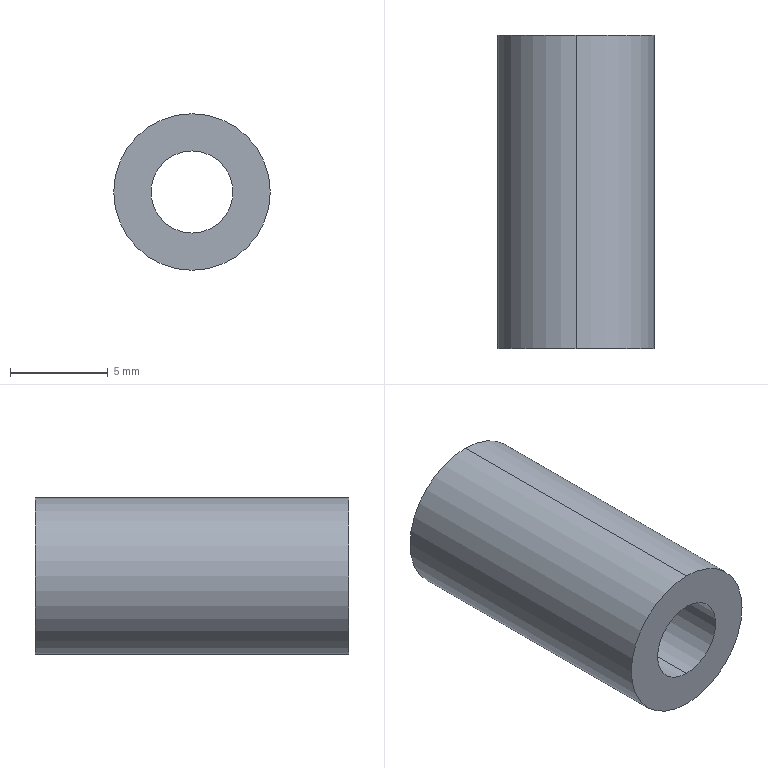Part | STEP file | 1 solid | 6 faces | box 8 x 16 x 8 mm | volume 582.577 mm3 | cylinder 4 | plane 2 | commonest cylinder face diameters 4.2 x2 8 x2
STEP:
#1=CARTESIAN_POINT('',(0.,0.,0.));
#2=DIRECTION('',(0.,0.,1.));
#3=DIRECTION('',(1.,0.,0.));
#4=AXIS2_PLACEMENT_3D('',#1,#2,#3);
#5=CARTESIAN_POINT('',(0.,16.,-2.1));
#6=VERTEX_POINT('',#5);
#7=CARTESIAN_POINT('',(0.,0.,-2.1));
#8=VERTEX_POINT('',#7);
#9=CARTESIAN_POINT('',(0.,16.,-2.1));
#10=DIRECTION('',(0.,-1.,0.));
#11=VECTOR('',#10,1.);
#12=LINE('',#9,#11);
#13=CARTESIAN_POINT('',(0.,16.,0.));
#14=DIRECTION('',(0.,-1.,0.));
#15=DIRECTION('',(0.,0.,-1.));
#16=AXIS2_PLACEMENT_3D('',#13,#14,#15);
#17=CYLINDRICAL_SURFACE('',#16,2.1);
#18=CARTESIAN_POINT('',(6.283,0.));
#19=DIRECTION('',(0.,1.));
#20=VECTOR('',#19,1.);
#21=LINE('',#18,#20);
#22=(GEOMETRIC_REPRESENTATION_CONTEXT(2)PARAMETRIC_REPRESENTATION_CONTEXT()REPRESENTATION_CONTEXT('',''));
#23=DEFINITIONAL_REPRESENTATION('',(#21),#22);
#24=PCURVE('',#17,#23);
#25=CARTESIAN_POINT('',(0.,16.,0.));
#26=DIRECTION('',(0.,-1.,0.));
#27=DIRECTION('',(0.,0.,-1.));
#28=AXIS2_PLACEMENT_3D('',#25,#26,#27);
#29=CYLINDRICAL_SURFACE('',#28,2.1);
#30=CARTESIAN_POINT('',(0.,0.));
#31=DIRECTION('',(0.,1.));
#32=VECTOR('',#31,1.);
#33=LINE('',#30,#32);
#34=(GEOMETRIC_REPRESENTATION_CONTEXT(2)PARAMETRIC_REPRESENTATION_CONTEXT()REPRESENTATION_CONTEXT('',''));
#35=DEFINITIONAL_REPRESENTATION('',(#33),#34);
#36=PCURVE('',#29,#35);
#37=SURFACE_CURVE('',#12,(#24,#36),.PCURVE_S1.);
#38=EDGE_CURVE('',#6,#8,#37,.T.);
#39=ORIENTED_EDGE('',*,*,#38,.T.);
#40=CARTESIAN_POINT('',(0.,0.,2.1));
#41=VERTEX_POINT('',#40);
#42=CARTESIAN_POINT('',(0.,0.,0.));
#43=DIRECTION('',(0.,1.,0.));
#44=DIRECTION('',(0.,0.,1.));
#45=AXIS2_PLACEMENT_3D('',#42,#43,#44);
#46=CIRCLE('',#45,2.1);
#47=CARTESIAN_POINT('',(9.425,16.));
#48=DIRECTION('',(-1.,0.));
#49=VECTOR('',#48,1.);
#50=LINE('',#47,#49);
#51=(GEOMETRIC_REPRESENTATION_CONTEXT(2)PARAMETRIC_REPRESENTATION_CONTEXT()REPRESENTATION_CONTEXT('',''));
#52=DEFINITIONAL_REPRESENTATION('',(#50),#51);
#53=PCURVE('',#17,#52);
#54=CARTESIAN_POINT('',(0.,0.,0.));
#55=DIRECTION('',(0.,1.,0.));
#56=DIRECTION('',(0.,0.,1.));
#57=AXIS2_PLACEMENT_3D('',#54,#55,#56);
#58=PLANE('',#57);
#59=CARTESIAN_POINT('',(0.,0.));
#60=DIRECTION('',(1.,0.));
#61=AXIS2_PLACEMENT_2D('',#59,#60);
#62=CIRCLE('',#61,2.1);
#63=(GEOMETRIC_REPRESENTATION_CONTEXT(2)PARAMETRIC_REPRESENTATION_CONTEXT()REPRESENTATION_CONTEXT('',''));
#64=DEFINITIONAL_REPRESENTATION('',(#62),#63);
#65=PCURVE('',#58,#64);
#66=SURFACE_CURVE('',#46,(#53,#65),.PCURVE_S1.);
#67=EDGE_CURVE('',#8,#41,#66,.T.);
#68=ORIENTED_EDGE('',*,*,#67,.T.);
#69=CARTESIAN_POINT('',(0.,16.,2.1));
#70=VERTEX_POINT('',#69);
#71=CARTESIAN_POINT('',(0.,16.,2.1));
#72=DIRECTION('',(0.,-1.,0.));
#73=VECTOR('',#72,1.);
#74=LINE('',#71,#73);
#75=CARTESIAN_POINT('',(3.142,0.));
#76=DIRECTION('',(0.,1.));
#77=VECTOR('',#76,1.);
#78=LINE('',#75,#77);
#79=(GEOMETRIC_REPRESENTATION_CONTEXT(2)PARAMETRIC_REPRESENTATION_CONTEXT()REPRESENTATION_CONTEXT('',''));
#80=DEFINITIONAL_REPRESENTATION('',(#78),#79);
#81=PCURVE('',#17,#80);
#82=CARTESIAN_POINT('',(3.142,0.));
#83=DIRECTION('',(0.,1.));
#84=VECTOR('',#83,1.);
#85=LINE('',#82,#84);
#86=(GEOMETRIC_REPRESENTATION_CONTEXT(2)PARAMETRIC_REPRESENTATION_CONTEXT()REPRESENTATION_CONTEXT('',''));
#87=DEFINITIONAL_REPRESENTATION('',(#85),#86);
#88=PCURVE('',#29,#87);
#89=SURFACE_CURVE('',#74,(#81,#88),.PCURVE_S1.);
#90=EDGE_CURVE('',#70,#41,#89,.T.);
#91=ORIENTED_EDGE('',*,*,#90,.F.);
#92=CARTESIAN_POINT('',(0.,16.,0.));
#93=DIRECTION('',(0.,1.,0.));
#94=DIRECTION('',(0.,0.,1.));
#95=AXIS2_PLACEMENT_3D('',#92,#93,#94);
#96=CIRCLE('',#95,2.1);
#97=CARTESIAN_POINT('',(9.425,0.));
#98=DIRECTION('',(-1.,0.));
#99=VECTOR('',#98,1.);
#100=LINE('',#97,#99);
#101=(GEOMETRIC_REPRESENTATION_CONTEXT(2)PARAMETRIC_REPRESENTATION_CONTEXT()REPRESENTATION_CONTEXT('',''));
#102=DEFINITIONAL_REPRESENTATION('',(#100),#101);
#103=PCURVE('',#17,#102);
#104=CARTESIAN_POINT('',(0.,16.,0.));
#105=DIRECTION('',(0.,1.,0.));
#106=DIRECTION('',(0.,0.,1.));
#107=AXIS2_PLACEMENT_3D('',#104,#105,#106);
#108=PLANE('',#107);
#109=CARTESIAN_POINT('',(0.,0.));
#110=DIRECTION('',(1.,0.));
#111=AXIS2_PLACEMENT_2D('',#109,#110);
#112=CIRCLE('',#111,2.1);
#113=(GEOMETRIC_REPRESENTATION_CONTEXT(2)PARAMETRIC_REPRESENTATION_CONTEXT()REPRESENTATION_CONTEXT('',''));
#114=DEFINITIONAL_REPRESENTATION('',(#112),#113);
#115=PCURVE('',#108,#114);
#116=SURFACE_CURVE('',#96,(#103,#115),.PCURVE_S1.);
#117=EDGE_CURVE('',#6,#70,#116,.T.);
#118=ORIENTED_EDGE('',*,*,#117,.F.);
#119=EDGE_LOOP('',(#39,#68,#91,#118));
#120=FACE_BOUND('',#119,.F.);
#121=ADVANCED_FACE('',(#120),#17,.F.);
#122=CARTESIAN_POINT('',(0.,16.,4.));
#123=VERTEX_POINT('',#122);
#124=CARTESIAN_POINT('',(0.,16.,-4.));
#125=VERTEX_POINT('',#124);
#126=CARTESIAN_POINT('',(0.,16.,0.));
#127=DIRECTION('',(0.,1.,0.));
#128=DIRECTION('',(0.,0.,1.));
#129=AXIS2_PLACEMENT_3D('',#126,#127,#128);
#130=CIRCLE('',#129,4.);
#131=CARTESIAN_POINT('',(0.,16.,0.));
#132=DIRECTION('',(0.,-1.,0.));
#133=DIRECTION('',(0.,0.,-1.));
#134=AXIS2_PLACEMENT_3D('',#131,#132,#133);
#135=CYLINDRICAL_SURFACE('',#134,4.);
#136=CARTESIAN_POINT('',(3.142,0.));
#137=DIRECTION('',(-1.,0.));
#138=VECTOR('',#137,1.);
#139=LINE('',#136,#138);
#140=(GEOMETRIC_REPRESENTATION_CONTEXT(2)PARAMETRIC_REPRESENTATION_CONTEXT()REPRESENTATION_CONTEXT('',''));
#141=DEFINITIONAL_REPRESENTATION('',(#139),#140);
#142=PCURVE('',#135,#141);
#143=CARTESIAN_POINT('',(0.,0.));
#144=DIRECTION('',(1.,0.));
#145=AXIS2_PLACEMENT_2D('',#143,#144);
#146=CIRCLE('',#145,4.);
#147=(GEOMETRIC_REPRESENTATION_CONTEXT(2)PARAMETRIC_REPRESENTATION_CONTEXT()REPRESENTATION_CONTEXT('',''));
#148=DEFINITIONAL_REPRESENTATION('',(#146),#147);
#149=PCURVE('',#108,#148);
#150=SURFACE_CURVE('',#130,(#142,#149),.PCURVE_S1.);
#151=EDGE_CURVE('',#123,#125,#150,.T.);
#152=ORIENTED_EDGE('',*,*,#151,.F.);
#153=CARTESIAN_POINT('',(0.,0.,4.));
#154=VERTEX_POINT('',#153);
#155=CARTESIAN_POINT('',(0.,16.,4.));
#156=DIRECTION('',(0.,-1.,0.));
#157=VECTOR('',#156,1.);
#158=LINE('',#155,#157);
#159=CARTESIAN_POINT('',(3.142,0.));
#160=DIRECTION('',(0.,1.));
#161=VECTOR('',#160,1.);
#162=LINE('',#159,#161);
#163=(GEOMETRIC_REPRESENTATION_CONTEXT(2)PARAMETRIC_REPRESENTATION_CONTEXT()REPRESENTATION_CONTEXT('',''));
#164=DEFINITIONAL_REPRESENTATION('',(#162),#163);
#165=PCURVE('',#135,#164);
#166=CARTESIAN_POINT('',(0.,16.,0.));
#167=DIRECTION('',(0.,-1.,0.));
#168=DIRECTION('',(0.,0.,-1.));
#169=AXIS2_PLACEMENT_3D('',#166,#167,#168);
#170=CYLINDRICAL_SURFACE('',#169,4.);
#171=CARTESIAN_POINT('',(3.142,0.));
#172=DIRECTION('',(0.,1.));
#173=VECTOR('',#172,1.);
#174=LINE('',#171,#173);
#175=(GEOMETRIC_REPRESENTATION_CONTEXT(2)PARAMETRIC_REPRESENTATION_CONTEXT()REPRESENTATION_CONTEXT('',''));
#176=DEFINITIONAL_REPRESENTATION('',(#174),#175);
#177=PCURVE('',#170,#176);
#178=SURFACE_CURVE('',#158,(#165,#177),.PCURVE_S1.);
#179=EDGE_CURVE('',#123,#154,#178,.T.);
#180=ORIENTED_EDGE('',*,*,#179,.T.);
#181=CARTESIAN_POINT('',(0.,0.,-4.));
#182=VERTEX_POINT('',#181);
#183=CARTESIAN_POINT('',(0.,0.,0.));
#184=DIRECTION('',(0.,1.,0.));
#185=DIRECTION('',(0.,0.,1.));
#186=AXIS2_PLACEMENT_3D('',#183,#184,#185);
#187=CIRCLE('',#186,4.);
#188=CARTESIAN_POINT('',(3.142,16.));
#189=DIRECTION('',(-1.,0.));
#190=VECTOR('',#189,1.);
#191=LINE('',#188,#190);
#192=(GEOMETRIC_REPRESENTATION_CONTEXT(2)PARAMETRIC_REPRESENTATION_CONTEXT()REPRESENTATION_CONTEXT('',''));
#193=DEFINITIONAL_REPRESENTATION('',(#191),#192);
#194=PCURVE('',#135,#193);
#195=CARTESIAN_POINT('',(0.,0.));
#196=DIRECTION('',(1.,0.));
#197=AXIS2_PLACEMENT_2D('',#195,#196);
#198=CIRCLE('',#197,4.);
#199=(GEOMETRIC_REPRESENTATION_CONTEXT(2)PARAMETRIC_REPRESENTATION_CONTEXT()REPRESENTATION_CONTEXT('',''));
#200=DEFINITIONAL_REPRESENTATION('',(#198),#199);
#201=PCURVE('',#58,#200);
#202=SURFACE_CURVE('',#187,(#194,#201),.PCURVE_S1.);
#203=EDGE_CURVE('',#154,#182,#202,.T.);
#204=ORIENTED_EDGE('',*,*,#203,.T.);
#205=CARTESIAN_POINT('',(0.,16.,-4.));
#206=DIRECTION('',(0.,-1.,0.));
#207=VECTOR('',#206,1.);
#208=LINE('',#205,#207);
#209=CARTESIAN_POINT('',(0.,0.));
#210=DIRECTION('',(0.,1.));
#211=VECTOR('',#210,1.);
#212=LINE('',#209,#211);
#213=(GEOMETRIC_REPRESENTATION_CONTEXT(2)PARAMETRIC_REPRESENTATION_CONTEXT()REPRESENTATION_CONTEXT('',''));
#214=DEFINITIONAL_REPRESENTATION('',(#212),#213);
#215=PCURVE('',#135,#214);
#216=CARTESIAN_POINT('',(6.283,0.));
#217=DIRECTION('',(0.,1.));
#218=VECTOR('',#217,1.);
#219=LINE('',#216,#218);
#220=(GEOMETRIC_REPRESENTATION_CONTEXT(2)PARAMETRIC_REPRESENTATION_CONTEXT()REPRESENTATION_CONTEXT('',''));
#221=DEFINITIONAL_REPRESENTATION('',(#219),#220);
#222=PCURVE('',#170,#221);
#223=SURFACE_CURVE('',#208,(#215,#222),.PCURVE_S1.);
#224=EDGE_CURVE('',#125,#182,#223,.T.);
#225=ORIENTED_EDGE('',*,*,#224,.F.);
#226=EDGE_LOOP('',(#152,#180,#204,#225));
#227=FACE_BOUND('',#226,.T.);
#228=ADVANCED_FACE('',(#227),#135,.T.);
#229=CARTESIAN_POINT('',(0.,16.,0.));
#230=DIRECTION('',(0.,1.,0.));
#231=DIRECTION('',(0.,0.,1.));
#232=AXIS2_PLACEMENT_3D('',#229,#230,#231);
#233=CIRCLE('',#232,4.);
#234=CARTESIAN_POINT('',(0.,0.));
#235=DIRECTION('',(1.,0.));
#236=AXIS2_PLACEMENT_2D('',#234,#235);
#237=CIRCLE('',#236,4.);
#238=(GEOMETRIC_REPRESENTATION_CONTEXT(2)PARAMETRIC_REPRESENTATION_CONTEXT()REPRESENTATION_CONTEXT('',''));
#239=DEFINITIONAL_REPRESENTATION('',(#237),#238);
#240=PCURVE('',#108,#239);
#241=CARTESIAN_POINT('',(9.425,0.));
#242=DIRECTION('',(-1.,0.));
#243=VECTOR('',#242,1.);
#244=LINE('',#241,#243);
#245=(GEOMETRIC_REPRESENTATION_CONTEXT(2)PARAMETRIC_REPRESENTATION_CONTEXT()REPRESENTATION_CONTEXT('',''));
#246=DEFINITIONAL_REPRESENTATION('',(#244),#245);
#247=PCURVE('',#170,#246);
#248=SURFACE_CURVE('',#233,(#240,#247),.PCURVE_S1.);
#249=EDGE_CURVE('',#125,#123,#248,.T.);
#250=ORIENTED_EDGE('',*,*,#249,.T.);
#251=ORIENTED_EDGE('',*,*,#151,.T.);
#252=EDGE_LOOP('',(#250,#251));
#253=FACE_BOUND('',#252,.T.);
#254=ORIENTED_EDGE('',*,*,#117,.F.);
#255=CARTESIAN_POINT('',(0.,16.,0.));
#256=DIRECTION('',(0.,1.,0.));
#257=DIRECTION('',(0.,0.,1.));
#258=AXIS2_PLACEMENT_3D('',#255,#256,#257);
#259=CIRCLE('',#258,2.1);
#260=CARTESIAN_POINT('',(0.,0.));
#261=DIRECTION('',(1.,0.));
#262=AXIS2_PLACEMENT_2D('',#260,#261);
#263=CIRCLE('',#262,2.1);
#264=(GEOMETRIC_REPRESENTATION_CONTEXT(2)PARAMETRIC_REPRESENTATION_CONTEXT()REPRESENTATION_CONTEXT('',''));
#265=DEFINITIONAL_REPRESENTATION('',(#263),#264);
#266=PCURVE('',#108,#265);
#267=CARTESIAN_POINT('',(3.142,0.));
#268=DIRECTION('',(-1.,0.));
#269=VECTOR('',#268,1.);
#270=LINE('',#267,#269);
#271=(GEOMETRIC_REPRESENTATION_CONTEXT(2)PARAMETRIC_REPRESENTATION_CONTEXT()REPRESENTATION_CONTEXT('',''));
#272=DEFINITIONAL_REPRESENTATION('',(#270),#271);
#273=PCURVE('',#29,#272);
#274=SURFACE_CURVE('',#259,(#266,#273),.PCURVE_S1.);
#275=EDGE_CURVE('',#70,#6,#274,.T.);
#276=ORIENTED_EDGE('',*,*,#275,.F.);
#277=EDGE_LOOP('',(#254,#276));
#278=FACE_BOUND('',#277,.T.);
#279=ADVANCED_FACE('',(#253,#278),#108,.T.);
#280=CARTESIAN_POINT('',(0.,0.,0.));
#281=DIRECTION('',(0.,1.,0.));
#282=DIRECTION('',(0.,0.,1.));
#283=AXIS2_PLACEMENT_3D('',#280,#281,#282);
#284=CIRCLE('',#283,4.);
#285=CARTESIAN_POINT('',(0.,0.));
#286=DIRECTION('',(1.,0.));
#287=AXIS2_PLACEMENT_2D('',#285,#286);
#288=CIRCLE('',#287,4.);
#289=(GEOMETRIC_REPRESENTATION_CONTEXT(2)PARAMETRIC_REPRESENTATION_CONTEXT()REPRESENTATION_CONTEXT('',''));
#290=DEFINITIONAL_REPRESENTATION('',(#288),#289);
#291=PCURVE('',#58,#290);
#292=CARTESIAN_POINT('',(9.425,16.));
#293=DIRECTION('',(-1.,0.));
#294=VECTOR('',#293,1.);
#295=LINE('',#292,#294);
#296=(GEOMETRIC_REPRESENTATION_CONTEXT(2)PARAMETRIC_REPRESENTATION_CONTEXT()REPRESENTATION_CONTEXT('',''));
#297=DEFINITIONAL_REPRESENTATION('',(#295),#296);
#298=PCURVE('',#170,#297);
#299=SURFACE_CURVE('',#284,(#291,#298),.PCURVE_S1.);
#300=EDGE_CURVE('',#182,#154,#299,.T.);
#301=ORIENTED_EDGE('',*,*,#300,.F.);
#302=ORIENTED_EDGE('',*,*,#203,.F.);
#303=EDGE_LOOP('',(#301,#302));
#304=FACE_BOUND('',#303,.T.);
#305=ORIENTED_EDGE('',*,*,#67,.T.);
#306=CARTESIAN_POINT('',(0.,0.,0.));
#307=DIRECTION('',(0.,1.,0.));
#308=DIRECTION('',(0.,0.,1.));
#309=AXIS2_PLACEMENT_3D('',#306,#307,#308);
#310=CIRCLE('',#309,2.1);
#311=CARTESIAN_POINT('',(0.,0.));
#312=DIRECTION('',(1.,0.));
#313=AXIS2_PLACEMENT_2D('',#311,#312);
#314=CIRCLE('',#313,2.1);
#315=(GEOMETRIC_REPRESENTATION_CONTEXT(2)PARAMETRIC_REPRESENTATION_CONTEXT()REPRESENTATION_CONTEXT('',''));
#316=DEFINITIONAL_REPRESENTATION('',(#314),#315);
#317=PCURVE('',#58,#316);
#318=CARTESIAN_POINT('',(3.142,16.));
#319=DIRECTION('',(-1.,0.));
#320=VECTOR('',#319,1.);
#321=LINE('',#318,#320);
#322=(GEOMETRIC_REPRESENTATION_CONTEXT(2)PARAMETRIC_REPRESENTATION_CONTEXT()REPRESENTATION_CONTEXT('',''));
#323=DEFINITIONAL_REPRESENTATION('',(#321),#322);
#324=PCURVE('',#29,#323);
#325=SURFACE_CURVE('',#310,(#317,#324),.PCURVE_S1.);
#326=EDGE_CURVE('',#41,#8,#325,.T.);
#327=ORIENTED_EDGE('',*,*,#326,.T.);
#328=EDGE_LOOP('',(#305,#327));
#329=FACE_BOUND('',#328,.T.);
#330=ADVANCED_FACE('',(#304,#329),#58,.F.);
#331=ORIENTED_EDGE('',*,*,#179,.F.);
#332=ORIENTED_EDGE('',*,*,#249,.F.);
#333=ORIENTED_EDGE('',*,*,#224,.T.);
#334=ORIENTED_EDGE('',*,*,#300,.T.);
#335=EDGE_LOOP('',(#331,#332,#333,#334));
#336=FACE_BOUND('',#335,.T.);
#337=ADVANCED_FACE('',(#336),#170,.T.);
#338=ORIENTED_EDGE('',*,*,#326,.T.);
#339=ORIENTED_EDGE('',*,*,#38,.F.);
#340=ORIENTED_EDGE('',*,*,#275,.F.);
#341=ORIENTED_EDGE('',*,*,#90,.T.);
#342=EDGE_LOOP('',(#338,#339,#340,#341));
#343=FACE_BOUND('',#342,.F.);
#344=ADVANCED_FACE('',(#343),#29,.F.);
#345=CLOSED_SHELL('',(#121,#228,#279,#330,#337,#344));
#346=MANIFOLD_SOLID_BREP('',#345);
#347=(LENGTH_UNIT()NAMED_UNIT(*)SI_UNIT(.MILLI.,.METRE.));
#348=UNCERTAINTY_MEASURE_WITH_UNIT(LENGTH_MEASURE(0.0000001),#347,'','');
#349=(NAMED_UNIT(*)PLANE_ANGLE_UNIT()SI_UNIT($,.RADIAN.));
#350=(NAMED_UNIT(*)SI_UNIT($,.STERADIAN.)SOLID_ANGLE_UNIT());
#351=(GEOMETRIC_REPRESENTATION_CONTEXT(3)GLOBAL_UNCERTAINTY_ASSIGNED_CONTEXT((#348))GLOBAL_UNIT_ASSIGNED_CONTEXT((#347,#349,#350))REPRESENTATION_CONTEXT('',''));
#352=ADVANCED_BREP_SHAPE_REPRESENTATION('',(#4,#346),#351);